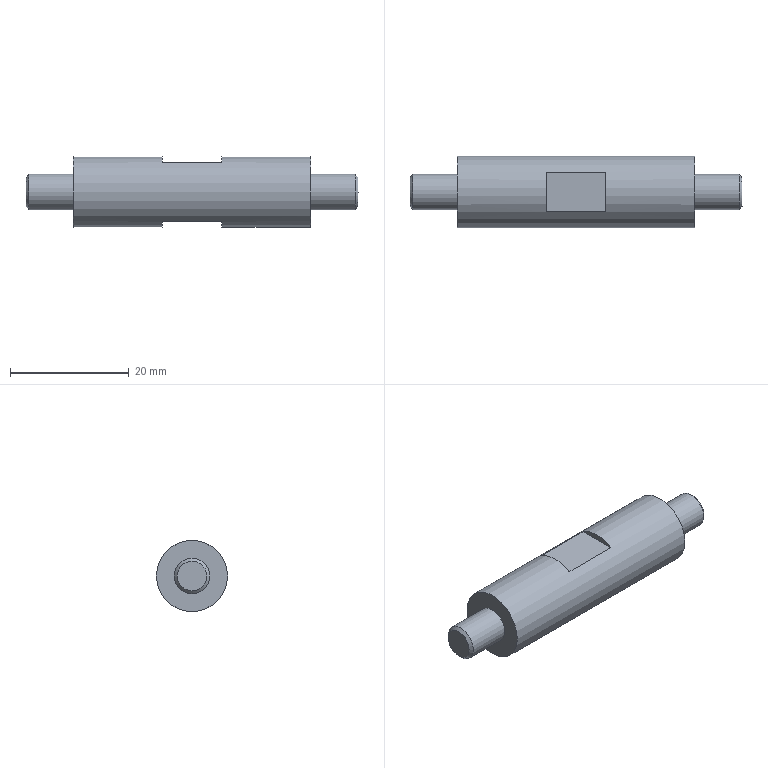Part | NX | features BREP 1 | 1 solid | 15 faces | box 56 x 12 x 12 mm | volume 4882 mm3 | plane 10 | cylinder 3 | cone 2 | commonest cylinder face diameters 6 x2 12 x1
STEP:
#1=CARTESIAN_POINT('',(20.,-6.,0.));
#2=VERTEX_POINT('',#1);
#3=CARTESIAN_POINT('',(20.,0.,0.));
#4=DIRECTION('',(-1.,0.,0.));
#5=DIRECTION('',(0.,-1.,0.));
#6=AXIS2_PLACEMENT_3D('',#3,#4,#5);
#7=CIRCLE('',#6,6.);
#8=EDGE_CURVE('',#2,#2,#7,.T.);
#9=ORIENTED_EDGE('',*,*,#8,.T.);
#10=EDGE_LOOP('',(#9));
#11=FACE_BOUND('',#10,.T.);
#12=CARTESIAN_POINT('',(-5.,-3.317,-5.));
#13=VERTEX_POINT('',#12);
#14=CARTESIAN_POINT('',(5.,-3.317,-5.));
#15=VERTEX_POINT('',#14);
#16=CARTESIAN_POINT('',(-28.,-3.317,-5.));
#17=DIRECTION('',(1.,0.,0.));
#18=VECTOR('',#17,1000.);
#19=LINE('',#16,#18);
#20=EDGE_CURVE('',#13,#15,#19,.T.);
#21=ORIENTED_EDGE('',*,*,#20,.T.);
#22=CARTESIAN_POINT('',(5.,3.317,-5.));
#23=VERTEX_POINT('',#22);
#24=CARTESIAN_POINT('',(5.,0.,0.));
#25=DIRECTION('',(1.,0.,0.));
#26=DIRECTION('',(0.,-1.,0.));
#27=AXIS2_PLACEMENT_3D('',#24,#25,#26);
#28=CIRCLE('',#27,6.);
#29=EDGE_CURVE('',#15,#23,#28,.T.);
#30=ORIENTED_EDGE('',*,*,#29,.T.);
#31=CARTESIAN_POINT('',(-5.,3.317,-5.));
#32=VERTEX_POINT('',#31);
#33=CARTESIAN_POINT('',(-28.,3.317,-5.));
#34=DIRECTION('',(-1.,0.,0.));
#35=VECTOR('',#34,1000.);
#36=LINE('',#33,#35);
#37=EDGE_CURVE('',#23,#32,#36,.T.);
#38=ORIENTED_EDGE('',*,*,#37,.T.);
#39=CARTESIAN_POINT('',(-5.,0.,0.));
#40=DIRECTION('',(-1.,0.,0.));
#41=DIRECTION('',(0.,-1.,0.));
#42=AXIS2_PLACEMENT_3D('',#39,#40,#41);
#43=CIRCLE('',#42,6.);
#44=EDGE_CURVE('',#32,#13,#43,.T.);
#45=ORIENTED_EDGE('',*,*,#44,.T.);
#46=EDGE_LOOP('',(#21,#30,#38,#45));
#47=FACE_BOUND('',#46,.T.);
#48=CARTESIAN_POINT('',(-20.,-6.,0.));
#49=VERTEX_POINT('',#48);
#50=CARTESIAN_POINT('',(-20.,0.,0.));
#51=DIRECTION('',(1.,0.,0.));
#52=DIRECTION('',(0.,-1.,0.));
#53=AXIS2_PLACEMENT_3D('',#50,#51,#52);
#54=CIRCLE('',#53,6.);
#55=EDGE_CURVE('',#49,#49,#54,.T.);
#56=ORIENTED_EDGE('',*,*,#55,.T.);
#57=EDGE_LOOP('',(#56));
#58=FACE_BOUND('',#57,.T.);
#59=CARTESIAN_POINT('',(5.,3.317,5.));
#60=VERTEX_POINT('',#59);
#61=CARTESIAN_POINT('',(5.,-3.317,5.));
#62=VERTEX_POINT('',#61);
#63=CARTESIAN_POINT('',(5.,0.,0.));
#64=DIRECTION('',(1.,0.,0.));
#65=DIRECTION('',(0.,-1.,0.));
#66=AXIS2_PLACEMENT_3D('',#63,#64,#65);
#67=CIRCLE('',#66,6.);
#68=EDGE_CURVE('',#60,#62,#67,.T.);
#69=ORIENTED_EDGE('',*,*,#68,.T.);
#70=CARTESIAN_POINT('',(-5.,-3.317,5.));
#71=VERTEX_POINT('',#70);
#72=CARTESIAN_POINT('',(-28.,-3.317,5.));
#73=DIRECTION('',(-1.,0.,0.));
#74=VECTOR('',#73,1000.);
#75=LINE('',#72,#74);
#76=EDGE_CURVE('',#62,#71,#75,.T.);
#77=ORIENTED_EDGE('',*,*,#76,.T.);
#78=CARTESIAN_POINT('',(-5.,3.317,5.));
#79=VERTEX_POINT('',#78);
#80=CARTESIAN_POINT('',(-5.,0.,0.));
#81=DIRECTION('',(-1.,0.,0.));
#82=DIRECTION('',(0.,-1.,0.));
#83=AXIS2_PLACEMENT_3D('',#80,#81,#82);
#84=CIRCLE('',#83,6.);
#85=EDGE_CURVE('',#71,#79,#84,.T.);
#86=ORIENTED_EDGE('',*,*,#85,.T.);
#87=CARTESIAN_POINT('',(-28.,3.317,5.));
#88=DIRECTION('',(1.,0.,0.));
#89=VECTOR('',#88,1000.);
#90=LINE('',#87,#89);
#91=EDGE_CURVE('',#79,#60,#90,.T.);
#92=ORIENTED_EDGE('',*,*,#91,.T.);
#93=EDGE_LOOP('',(#69,#77,#86,#92));
#94=FACE_BOUND('',#93,.T.);
#95=CARTESIAN_POINT('',(-28.,0.,0.));
#96=DIRECTION('',(-1.,0.,0.));
#97=DIRECTION('',(0.,1.,0.));
#98=AXIS2_PLACEMENT_3D('',#95,#96,#97);
#99=CYLINDRICAL_SURFACE('',#98,6.);
#100=ADVANCED_FACE('',(#11,#47,#58,#94),#99,.T.);
#101=ORIENTED_EDGE('',*,*,#29,.F.);
#102=CARTESIAN_POINT('',(5.,0.,-5.));
#103=DIRECTION('',(0.,1.,0.));
#104=VECTOR('',#103,1000.);
#105=LINE('',#102,#104);
#106=EDGE_CURVE('',#15,#23,#105,.T.);
#107=ORIENTED_EDGE('',*,*,#106,.T.);
#108=EDGE_LOOP('',(#101,#107));
#109=FACE_BOUND('',#108,.T.);
#110=CARTESIAN_POINT('',(5.,0.,0.));
#111=DIRECTION('',(-1.,0.,0.));
#112=DIRECTION('',(0.,0.,-1.));
#113=AXIS2_PLACEMENT_3D('',#110,#111,#112);
#114=PLANE('',#113);
#115=ADVANCED_FACE('',(#109),#114,.T.);
#116=ORIENTED_EDGE('',*,*,#20,.F.);
#117=CARTESIAN_POINT('',(-5.,6.286,-5.));
#118=DIRECTION('',(0.,-1.,0.));
#119=VECTOR('',#118,1000.);
#120=LINE('',#117,#119);
#121=EDGE_CURVE('',#32,#13,#120,.T.);
#122=ORIENTED_EDGE('',*,*,#121,.F.);
#123=ORIENTED_EDGE('',*,*,#37,.F.);
#124=ORIENTED_EDGE('',*,*,#106,.F.);
#125=EDGE_LOOP('',(#116,#122,#123,#124));
#126=FACE_BOUND('',#125,.T.);
#127=CARTESIAN_POINT('',(-5.,6.286,-5.));
#128=DIRECTION('',(0.,0.,1.));
#129=DIRECTION('',(-1.,0.,0.));
#130=AXIS2_PLACEMENT_3D('',#127,#128,#129);
#131=PLANE('',#130);
#132=ADVANCED_FACE('',(#126),#131,.F.);
#133=ORIENTED_EDGE('',*,*,#44,.F.);
#134=ORIENTED_EDGE('',*,*,#121,.T.);
#135=EDGE_LOOP('',(#133,#134));
#136=FACE_BOUND('',#135,.T.);
#137=CARTESIAN_POINT('',(-5.,0.,0.));
#138=DIRECTION('',(-1.,0.,0.));
#139=DIRECTION('',(0.,0.,-1.));
#140=AXIS2_PLACEMENT_3D('',#137,#138,#139);
#141=PLANE('',#140);
#142=ADVANCED_FACE('',(#136),#141,.F.);
#143=ORIENTED_EDGE('',*,*,#55,.F.);
#144=EDGE_LOOP('',(#143));
#145=FACE_BOUND('',#144,.T.);
#146=CARTESIAN_POINT('',(-20.,-3.,0.));
#147=VERTEX_POINT('',#146);
#148=CARTESIAN_POINT('',(-20.,0.,0.));
#149=DIRECTION('',(-1.,0.,0.));
#150=DIRECTION('',(0.,-1.,0.));
#151=AXIS2_PLACEMENT_3D('',#148,#149,#150);
#152=CIRCLE('',#151,3.);
#153=EDGE_CURVE('',#147,#147,#152,.T.);
#154=ORIENTED_EDGE('',*,*,#153,.F.);
#155=EDGE_LOOP('',(#154));
#156=FACE_BOUND('',#155,.T.);
#157=CARTESIAN_POINT('',(-20.,6.,0.));
#158=DIRECTION('',(1.,0.,0.));
#159=DIRECTION('',(0.,-1.,0.));
#160=AXIS2_PLACEMENT_3D('',#157,#158,#159);
#161=PLANE('',#160);
#162=ADVANCED_FACE('',(#145,#156),#161,.F.);
#163=CARTESIAN_POINT('',(20.,-3.,0.));
#164=VERTEX_POINT('',#163);
#165=CARTESIAN_POINT('',(20.,0.,0.));
#166=DIRECTION('',(1.,0.,0.));
#167=DIRECTION('',(0.,-1.,0.));
#168=AXIS2_PLACEMENT_3D('',#165,#166,#167);
#169=CIRCLE('',#168,3.);
#170=EDGE_CURVE('',#164,#164,#169,.T.);
#171=ORIENTED_EDGE('',*,*,#170,.F.);
#172=EDGE_LOOP('',(#171));
#173=FACE_BOUND('',#172,.T.);
#174=ORIENTED_EDGE('',*,*,#8,.F.);
#175=EDGE_LOOP('',(#174));
#176=FACE_BOUND('',#175,.T.);
#177=CARTESIAN_POINT('',(20.,3.,0.));
#178=DIRECTION('',(-1.,0.,0.));
#179=DIRECTION('',(0.,1.,0.));
#180=AXIS2_PLACEMENT_3D('',#177,#178,#179);
#181=PLANE('',#180);
#182=ADVANCED_FACE('',(#173,#176),#181,.F.);
#183=CARTESIAN_POINT('',(-27.5,-3.,0.));
#184=VERTEX_POINT('',#183);
#185=CARTESIAN_POINT('',(-27.5,0.,0.));
#186=DIRECTION('',(1.,0.,0.));
#187=DIRECTION('',(0.,-1.,0.));
#188=AXIS2_PLACEMENT_3D('',#185,#186,#187);
#189=CIRCLE('',#188,3.);
#190=EDGE_CURVE('',#184,#184,#189,.T.);
#191=ORIENTED_EDGE('',*,*,#190,.T.);
#192=EDGE_LOOP('',(#191));
#193=FACE_BOUND('',#192,.T.);
#194=ORIENTED_EDGE('',*,*,#153,.T.);
#195=EDGE_LOOP('',(#194));
#196=FACE_BOUND('',#195,.T.);
#197=CARTESIAN_POINT('',(-28.,0.,0.));
#198=DIRECTION('',(-1.,0.,0.));
#199=DIRECTION('',(0.,1.,0.));
#200=AXIS2_PLACEMENT_3D('',#197,#198,#199);
#201=CYLINDRICAL_SURFACE('',#200,3.);
#202=ADVANCED_FACE('',(#193,#196),#201,.T.);
#203=ORIENTED_EDGE('',*,*,#91,.F.);
#204=CARTESIAN_POINT('',(-5.,6.286,5.));
#205=DIRECTION('',(0.,1.,0.));
#206=VECTOR('',#205,1000.);
#207=LINE('',#204,#206);
#208=EDGE_CURVE('',#71,#79,#207,.T.);
#209=ORIENTED_EDGE('',*,*,#208,.F.);
#210=ORIENTED_EDGE('',*,*,#76,.F.);
#211=CARTESIAN_POINT('',(5.,6.286,5.));
#212=DIRECTION('',(0.,-1.,0.));
#213=VECTOR('',#212,1000.);
#214=LINE('',#211,#213);
#215=EDGE_CURVE('',#60,#62,#214,.T.);
#216=ORIENTED_EDGE('',*,*,#215,.F.);
#217=EDGE_LOOP('',(#203,#209,#210,#216));
#218=FACE_BOUND('',#217,.T.);
#219=CARTESIAN_POINT('',(-5.,6.286,5.));
#220=DIRECTION('',(0.,0.,-1.));
#221=DIRECTION('',(1.,0.,0.));
#222=AXIS2_PLACEMENT_3D('',#219,#220,#221);
#223=PLANE('',#222);
#224=ADVANCED_FACE('',(#218),#223,.F.);
#225=ORIENTED_EDGE('',*,*,#68,.F.);
#226=ORIENTED_EDGE('',*,*,#215,.T.);
#227=EDGE_LOOP('',(#225,#226));
#228=FACE_BOUND('',#227,.T.);
#229=CARTESIAN_POINT('',(5.,0.,0.));
#230=DIRECTION('',(1.,0.,0.));
#231=DIRECTION('',(0.,0.,1.));
#232=AXIS2_PLACEMENT_3D('',#229,#230,#231);
#233=PLANE('',#232);
#234=ADVANCED_FACE('',(#228),#233,.F.);
#235=ORIENTED_EDGE('',*,*,#85,.F.);
#236=ORIENTED_EDGE('',*,*,#208,.T.);
#237=EDGE_LOOP('',(#235,#236));
#238=FACE_BOUND('',#237,.T.);
#239=CARTESIAN_POINT('',(-5.,0.,0.));
#240=DIRECTION('',(1.,0.,0.));
#241=DIRECTION('',(0.,0.,1.));
#242=AXIS2_PLACEMENT_3D('',#239,#240,#241);
#243=PLANE('',#242);
#244=ADVANCED_FACE('',(#238),#243,.T.);
#245=ORIENTED_EDGE('',*,*,#170,.T.);
#246=EDGE_LOOP('',(#245));
#247=FACE_BOUND('',#246,.T.);
#248=CARTESIAN_POINT('',(27.5,-3.,0.));
#249=VERTEX_POINT('',#248);
#250=CARTESIAN_POINT('',(27.5,0.,0.));
#251=DIRECTION('',(-1.,0.,0.));
#252=DIRECTION('',(0.,-1.,0.));
#253=AXIS2_PLACEMENT_3D('',#250,#251,#252);
#254=CIRCLE('',#253,3.);
#255=EDGE_CURVE('',#249,#249,#254,.T.);
#256=ORIENTED_EDGE('',*,*,#255,.T.);
#257=EDGE_LOOP('',(#256));
#258=FACE_BOUND('',#257,.T.);
#259=CARTESIAN_POINT('',(-28.,0.,0.));
#260=DIRECTION('',(-1.,0.,0.));
#261=DIRECTION('',(0.,1.,0.));
#262=AXIS2_PLACEMENT_3D('',#259,#260,#261);
#263=CYLINDRICAL_SURFACE('',#262,3.);
#264=ADVANCED_FACE('',(#247,#258),#263,.T.);
#265=ORIENTED_EDGE('',*,*,#190,.F.);
#266=EDGE_LOOP('',(#265));
#267=FACE_BOUND('',#266,.T.);
#268=CARTESIAN_POINT('',(-28.,0.,-2.5));
#269=VERTEX_POINT('',#268);
#270=CARTESIAN_POINT('',(-28.,0.,0.));
#271=DIRECTION('',(1.,0.,0.));
#272=DIRECTION('',(0.,0.,-1.));
#273=AXIS2_PLACEMENT_3D('',#270,#271,#272);
#274=CIRCLE('',#273,2.5);
#275=EDGE_CURVE('',#269,#269,#274,.T.);
#276=ORIENTED_EDGE('',*,*,#275,.T.);
#277=EDGE_LOOP('',(#276));
#278=FACE_BOUND('',#277,.T.);
#279=CARTESIAN_POINT('',(-27.5,0.,0.));
#280=DIRECTION('',(1.,0.,0.));
#281=DIRECTION('',(0.,0.,1.));
#282=AXIS2_PLACEMENT_3D('',#279,#280,#281);
#283=CONICAL_SURFACE('',#282,3.,0.7854);
#284=ADVANCED_FACE('',(#267,#278),#283,.T.);
#285=ORIENTED_EDGE('',*,*,#255,.F.);
#286=EDGE_LOOP('',(#285));
#287=FACE_BOUND('',#286,.T.);
#288=CARTESIAN_POINT('',(28.,0.,2.5));
#289=VERTEX_POINT('',#288);
#290=CARTESIAN_POINT('',(28.,0.,0.));
#291=DIRECTION('',(-1.,0.,0.));
#292=DIRECTION('',(0.,0.,1.));
#293=AXIS2_PLACEMENT_3D('',#290,#291,#292);
#294=CIRCLE('',#293,2.5);
#295=EDGE_CURVE('',#289,#289,#294,.T.);
#296=ORIENTED_EDGE('',*,*,#295,.T.);
#297=EDGE_LOOP('',(#296));
#298=FACE_BOUND('',#297,.T.);
#299=CARTESIAN_POINT('',(27.5,0.,0.));
#300=DIRECTION('',(-1.,0.,0.));
#301=DIRECTION('',(0.,0.,-1.));
#302=AXIS2_PLACEMENT_3D('',#299,#300,#301);
#303=CONICAL_SURFACE('',#302,3.,0.7854);
#304=ADVANCED_FACE('',(#287,#298),#303,.T.);
#305=ORIENTED_EDGE('',*,*,#275,.F.);
#306=EDGE_LOOP('',(#305));
#307=FACE_BOUND('',#306,.T.);
#308=CARTESIAN_POINT('',(-28.,3.,0.));
#309=DIRECTION('',(1.,0.,0.));
#310=DIRECTION('',(0.,-1.,0.));
#311=AXIS2_PLACEMENT_3D('',#308,#309,#310);
#312=PLANE('',#311);
#313=ADVANCED_FACE('',(#307),#312,.F.);
#314=ORIENTED_EDGE('',*,*,#295,.F.);
#315=EDGE_LOOP('',(#314));
#316=FACE_BOUND('',#315,.T.);
#317=CARTESIAN_POINT('',(28.,0.,0.));
#318=DIRECTION('',(-1.,0.,0.));
#319=DIRECTION('',(0.,1.,0.));
#320=AXIS2_PLACEMENT_3D('',#317,#318,#319);
#321=PLANE('',#320);
#322=ADVANCED_FACE('',(#316),#321,.F.);
#323=CLOSED_SHELL('',(#100,#115,#132,#142,#162,#182,#202,#224,#234,#244,#264,#284,#304,#313,#322));
#324=MANIFOLD_SOLID_BREP('',#323);
#325=(LENGTH_UNIT()NAMED_UNIT(*)SI_UNIT(.MILLI.,.METRE.));
#326=UNCERTAINTY_MEASURE_WITH_UNIT(LENGTH_MEASURE(0.00001),#325,'','');
#327=(NAMED_UNIT(*)PLANE_ANGLE_UNIT()SI_UNIT($,.RADIAN.));
#328=(NAMED_UNIT(*)SI_UNIT($,.STERADIAN.)SOLID_ANGLE_UNIT());
#329=(GEOMETRIC_REPRESENTATION_CONTEXT(3)GLOBAL_UNCERTAINTY_ASSIGNED_CONTEXT((#326))GLOBAL_UNIT_ASSIGNED_CONTEXT((#325,#327,#328))REPRESENTATION_CONTEXT('',''));
#330=ADVANCED_BREP_SHAPE_REPRESENTATION('',(#324),#329);